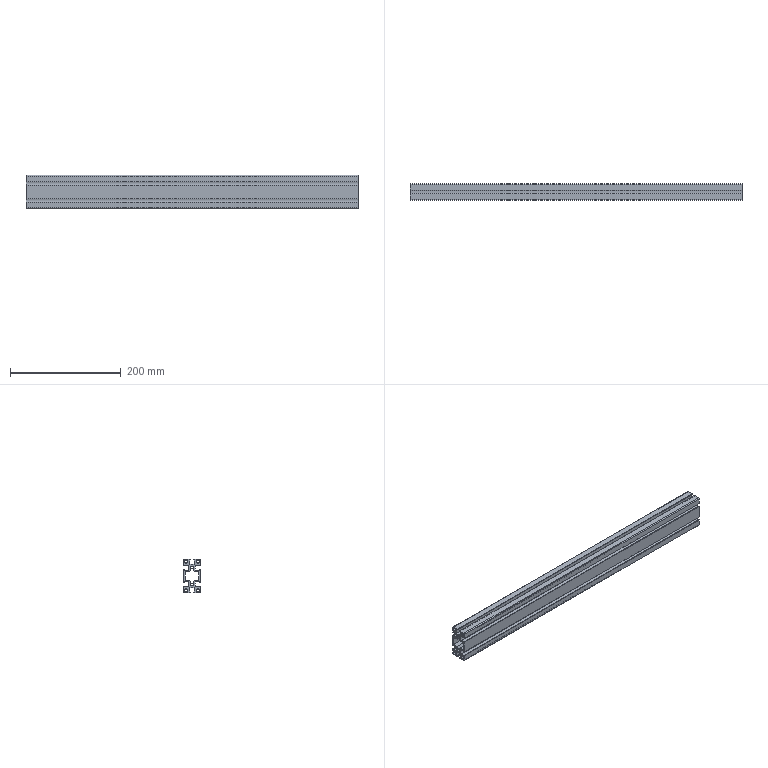Part | SolidWorks | features WeldMemberFeat 1, WeldmentFeature 1 | 1 solid | 84 faces | box 600 x 30 x 60 mm | volume 465086 mm3 | plane 58 | cylinder 26 | commonest cylinder face diameters 5.3 x8 24 x8 5 x6 3 x4